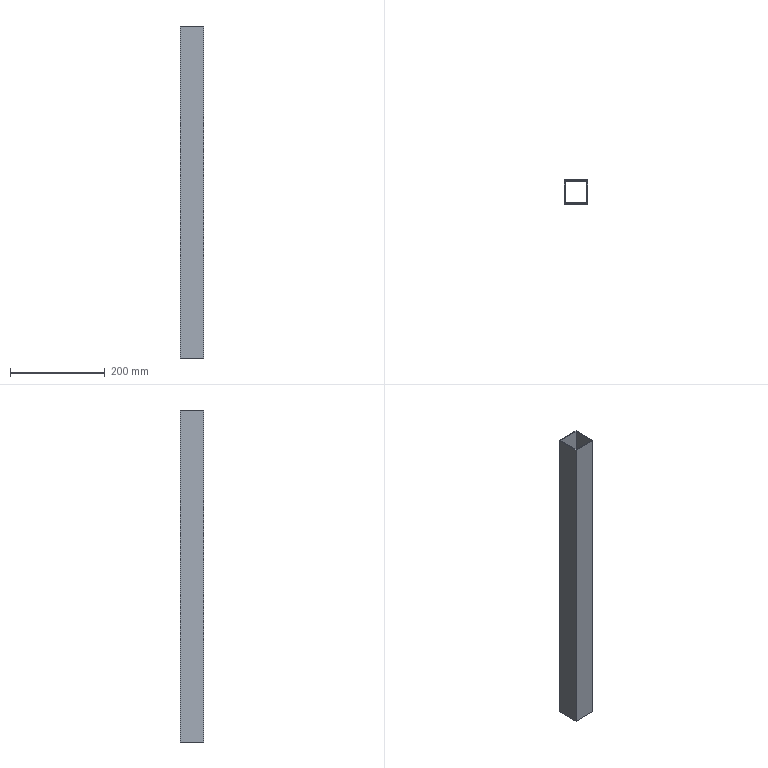Part | SolidWorks | features Extrusion 1 | 1 solid | 10 faces | box 50 x 50 x 700 mm | volume 268800 mm3 | plane 10
STEP:
#1=CARTESIAN_POINT('',(25.,-25.,700.));
#2=VERTEX_POINT('',#1);
#3=CARTESIAN_POINT('',(25.,25.,700.));
#4=VERTEX_POINT('',#3);
#5=CARTESIAN_POINT('',(25.,-25.,700.));
#6=DIRECTION('',(0.,1.,0.));
#7=VECTOR('',#6,1000.);
#8=LINE('',#5,#7);
#9=EDGE_CURVE('',#2,#4,#8,.T.);
#10=ORIENTED_EDGE('',*,*,#9,.T.);
#11=CARTESIAN_POINT('',(-25.,25.,700.));
#12=VERTEX_POINT('',#11);
#13=CARTESIAN_POINT('',(-25.,25.,700.));
#14=DIRECTION('',(-1.,0.,0.));
#15=VECTOR('',#14,1000.);
#16=LINE('',#13,#15);
#17=EDGE_CURVE('',#4,#12,#16,.T.);
#18=ORIENTED_EDGE('',*,*,#17,.T.);
#19=CARTESIAN_POINT('',(-25.,-25.,700.));
#20=VERTEX_POINT('',#19);
#21=CARTESIAN_POINT('',(-25.,-25.,700.));
#22=DIRECTION('',(0.,-1.,0.));
#23=VECTOR('',#22,1000.);
#24=LINE('',#21,#23);
#25=EDGE_CURVE('',#12,#20,#24,.T.);
#26=ORIENTED_EDGE('',*,*,#25,.T.);
#27=CARTESIAN_POINT('',(-25.,-25.,700.));
#28=DIRECTION('',(1.,0.,0.));
#29=VECTOR('',#28,1000.);
#30=LINE('',#27,#29);
#31=EDGE_CURVE('',#20,#2,#30,.T.);
#32=ORIENTED_EDGE('',*,*,#31,.T.);
#33=EDGE_LOOP('',(#10,#18,#26,#32));
#34=FACE_OUTER_BOUND('',#33,.T.);
#35=CARTESIAN_POINT('',(23.,-23.,700.));
#36=VERTEX_POINT('',#35);
#37=CARTESIAN_POINT('',(23.,23.,700.));
#38=VERTEX_POINT('',#37);
#39=CARTESIAN_POINT('',(23.,-23.,700.));
#40=DIRECTION('',(0.,1.,0.));
#41=VECTOR('',#40,1000.);
#42=LINE('',#39,#41);
#43=EDGE_CURVE('',#36,#38,#42,.T.);
#44=ORIENTED_EDGE('',*,*,#43,.F.);
#45=CARTESIAN_POINT('',(-23.,-23.,700.));
#46=VERTEX_POINT('',#45);
#47=CARTESIAN_POINT('',(-23.,-23.,700.));
#48=DIRECTION('',(1.,0.,0.));
#49=VECTOR('',#48,1000.);
#50=LINE('',#47,#49);
#51=EDGE_CURVE('',#46,#36,#50,.T.);
#52=ORIENTED_EDGE('',*,*,#51,.F.);
#53=CARTESIAN_POINT('',(-23.,23.,700.));
#54=VERTEX_POINT('',#53);
#55=CARTESIAN_POINT('',(-23.,-23.,700.));
#56=DIRECTION('',(0.,-1.,0.));
#57=VECTOR('',#56,1000.);
#58=LINE('',#55,#57);
#59=EDGE_CURVE('',#54,#46,#58,.T.);
#60=ORIENTED_EDGE('',*,*,#59,.F.);
#61=CARTESIAN_POINT('',(-23.,23.,700.));
#62=DIRECTION('',(-1.,0.,0.));
#63=VECTOR('',#62,1000.);
#64=LINE('',#61,#63);
#65=EDGE_CURVE('',#38,#54,#64,.T.);
#66=ORIENTED_EDGE('',*,*,#65,.F.);
#67=EDGE_LOOP('',(#44,#52,#60,#66));
#68=FACE_BOUND('',#67,.T.);
#69=CARTESIAN_POINT('',(0.,0.,700.));
#70=DIRECTION('',(0.,0.,-1.));
#71=DIRECTION('',(-1.,0.,0.));
#72=AXIS2_PLACEMENT_3D('',#69,#70,#71);
#73=PLANE('',#72);
#74=ADVANCED_FACE('',(#34,#68),#73,.F.);
#75=CARTESIAN_POINT('',(25.,-25.,0.));
#76=VERTEX_POINT('',#75);
#77=CARTESIAN_POINT('',(25.,25.,0.));
#78=VERTEX_POINT('',#77);
#79=CARTESIAN_POINT('',(25.,-25.,0.));
#80=DIRECTION('',(0.,1.,0.));
#81=VECTOR('',#80,1000.);
#82=LINE('',#79,#81);
#83=EDGE_CURVE('',#76,#78,#82,.T.);
#84=ORIENTED_EDGE('',*,*,#83,.F.);
#85=CARTESIAN_POINT('',(-25.,-25.,0.));
#86=VERTEX_POINT('',#85);
#87=CARTESIAN_POINT('',(-25.,-25.,0.));
#88=DIRECTION('',(1.,0.,0.));
#89=VECTOR('',#88,1000.);
#90=LINE('',#87,#89);
#91=EDGE_CURVE('',#86,#76,#90,.T.);
#92=ORIENTED_EDGE('',*,*,#91,.F.);
#93=CARTESIAN_POINT('',(-25.,25.,0.));
#94=VERTEX_POINT('',#93);
#95=CARTESIAN_POINT('',(-25.,-25.,0.));
#96=DIRECTION('',(0.,-1.,0.));
#97=VECTOR('',#96,1000.);
#98=LINE('',#95,#97);
#99=EDGE_CURVE('',#94,#86,#98,.T.);
#100=ORIENTED_EDGE('',*,*,#99,.F.);
#101=CARTESIAN_POINT('',(-25.,25.,0.));
#102=DIRECTION('',(-1.,0.,0.));
#103=VECTOR('',#102,1000.);
#104=LINE('',#101,#103);
#105=EDGE_CURVE('',#78,#94,#104,.T.);
#106=ORIENTED_EDGE('',*,*,#105,.F.);
#107=EDGE_LOOP('',(#84,#92,#100,#106));
#108=FACE_OUTER_BOUND('',#107,.T.);
#109=CARTESIAN_POINT('',(-23.,-23.,0.));
#110=VERTEX_POINT('',#109);
#111=CARTESIAN_POINT('',(23.,-23.,0.));
#112=VERTEX_POINT('',#111);
#113=CARTESIAN_POINT('',(-23.,-23.,0.));
#114=DIRECTION('',(1.,0.,0.));
#115=VECTOR('',#114,1000.);
#116=LINE('',#113,#115);
#117=EDGE_CURVE('',#110,#112,#116,.T.);
#118=ORIENTED_EDGE('',*,*,#117,.T.);
#119=CARTESIAN_POINT('',(23.,23.,0.));
#120=VERTEX_POINT('',#119);
#121=CARTESIAN_POINT('',(23.,-23.,0.));
#122=DIRECTION('',(0.,1.,0.));
#123=VECTOR('',#122,1000.);
#124=LINE('',#121,#123);
#125=EDGE_CURVE('',#112,#120,#124,.T.);
#126=ORIENTED_EDGE('',*,*,#125,.T.);
#127=CARTESIAN_POINT('',(-23.,23.,0.));
#128=VERTEX_POINT('',#127);
#129=CARTESIAN_POINT('',(-23.,23.,0.));
#130=DIRECTION('',(-1.,0.,0.));
#131=VECTOR('',#130,1000.);
#132=LINE('',#129,#131);
#133=EDGE_CURVE('',#120,#128,#132,.T.);
#134=ORIENTED_EDGE('',*,*,#133,.T.);
#135=CARTESIAN_POINT('',(-23.,-23.,0.));
#136=DIRECTION('',(0.,-1.,0.));
#137=VECTOR('',#136,1000.);
#138=LINE('',#135,#137);
#139=EDGE_CURVE('',#128,#110,#138,.T.);
#140=ORIENTED_EDGE('',*,*,#139,.T.);
#141=EDGE_LOOP('',(#118,#126,#134,#140));
#142=FACE_BOUND('',#141,.T.);
#143=CARTESIAN_POINT('',(0.,0.,0.));
#144=DIRECTION('',(0.,0.,-1.));
#145=DIRECTION('',(-1.,0.,0.));
#146=AXIS2_PLACEMENT_3D('',#143,#144,#145);
#147=PLANE('',#146);
#148=ADVANCED_FACE('',(#108,#142),#147,.T.);
#149=ORIENTED_EDGE('',*,*,#83,.T.);
#150=CARTESIAN_POINT('',(25.,25.,700.));
#151=DIRECTION('',(0.,0.,-1.));
#152=VECTOR('',#151,1000.);
#153=LINE('',#150,#152);
#154=EDGE_CURVE('',#4,#78,#153,.T.);
#155=ORIENTED_EDGE('',*,*,#154,.F.);
#156=ORIENTED_EDGE('',*,*,#9,.F.);
#157=CARTESIAN_POINT('',(25.,-25.,700.));
#158=DIRECTION('',(0.,0.,-1.));
#159=VECTOR('',#158,1000.);
#160=LINE('',#157,#159);
#161=EDGE_CURVE('',#2,#76,#160,.T.);
#162=ORIENTED_EDGE('',*,*,#161,.T.);
#163=EDGE_LOOP('',(#149,#155,#156,#162));
#164=FACE_OUTER_BOUND('',#163,.T.);
#165=CARTESIAN_POINT('',(25.,-25.,700.));
#166=DIRECTION('',(-1.,0.,0.));
#167=DIRECTION('',(0.,0.,1.));
#168=AXIS2_PLACEMENT_3D('',#165,#166,#167);
#169=PLANE('',#168);
#170=ADVANCED_FACE('',(#164),#169,.F.);
#171=ORIENTED_EDGE('',*,*,#105,.T.);
#172=CARTESIAN_POINT('',(-25.,25.,700.));
#173=DIRECTION('',(0.,0.,-1.));
#174=VECTOR('',#173,1000.);
#175=LINE('',#172,#174);
#176=EDGE_CURVE('',#12,#94,#175,.T.);
#177=ORIENTED_EDGE('',*,*,#176,.F.);
#178=ORIENTED_EDGE('',*,*,#17,.F.);
#179=ORIENTED_EDGE('',*,*,#154,.T.);
#180=EDGE_LOOP('',(#171,#177,#178,#179));
#181=FACE_OUTER_BOUND('',#180,.T.);
#182=CARTESIAN_POINT('',(-25.,25.,700.));
#183=DIRECTION('',(0.,-1.,0.));
#184=DIRECTION('',(0.,0.,-1.));
#185=AXIS2_PLACEMENT_3D('',#182,#183,#184);
#186=PLANE('',#185);
#187=ADVANCED_FACE('',(#181),#186,.F.);
#188=ORIENTED_EDGE('',*,*,#99,.T.);
#189=CARTESIAN_POINT('',(-25.,-25.,700.));
#190=DIRECTION('',(0.,0.,-1.));
#191=VECTOR('',#190,1000.);
#192=LINE('',#189,#191);
#193=EDGE_CURVE('',#20,#86,#192,.T.);
#194=ORIENTED_EDGE('',*,*,#193,.F.);
#195=ORIENTED_EDGE('',*,*,#25,.F.);
#196=ORIENTED_EDGE('',*,*,#176,.T.);
#197=EDGE_LOOP('',(#188,#194,#195,#196));
#198=FACE_OUTER_BOUND('',#197,.T.);
#199=CARTESIAN_POINT('',(-25.,-25.,700.));
#200=DIRECTION('',(1.,0.,0.));
#201=DIRECTION('',(0.,0.,-1.));
#202=AXIS2_PLACEMENT_3D('',#199,#200,#201);
#203=PLANE('',#202);
#204=ADVANCED_FACE('',(#198),#203,.F.);
#205=ORIENTED_EDGE('',*,*,#91,.T.);
#206=ORIENTED_EDGE('',*,*,#161,.F.);
#207=ORIENTED_EDGE('',*,*,#31,.F.);
#208=ORIENTED_EDGE('',*,*,#193,.T.);
#209=EDGE_LOOP('',(#205,#206,#207,#208));
#210=FACE_OUTER_BOUND('',#209,.T.);
#211=CARTESIAN_POINT('',(-25.,-25.,700.));
#212=DIRECTION('',(0.,1.,0.));
#213=DIRECTION('',(0.,0.,1.));
#214=AXIS2_PLACEMENT_3D('',#211,#212,#213);
#215=PLANE('',#214);
#216=ADVANCED_FACE('',(#210),#215,.F.);
#217=ORIENTED_EDGE('',*,*,#125,.F.);
#218=CARTESIAN_POINT('',(23.,-23.,700.));
#219=DIRECTION('',(0.,0.,-1.));
#220=VECTOR('',#219,1000.);
#221=LINE('',#218,#220);
#222=EDGE_CURVE('',#36,#112,#221,.T.);
#223=ORIENTED_EDGE('',*,*,#222,.F.);
#224=ORIENTED_EDGE('',*,*,#43,.T.);
#225=CARTESIAN_POINT('',(23.,23.,700.));
#226=DIRECTION('',(0.,0.,-1.));
#227=VECTOR('',#226,1000.);
#228=LINE('',#225,#227);
#229=EDGE_CURVE('',#38,#120,#228,.T.);
#230=ORIENTED_EDGE('',*,*,#229,.T.);
#231=EDGE_LOOP('',(#217,#223,#224,#230));
#232=FACE_OUTER_BOUND('',#231,.T.);
#233=CARTESIAN_POINT('',(23.,-23.,700.));
#234=DIRECTION('',(-1.,0.,0.));
#235=DIRECTION('',(0.,0.,1.));
#236=AXIS2_PLACEMENT_3D('',#233,#234,#235);
#237=PLANE('',#236);
#238=ADVANCED_FACE('',(#232),#237,.T.);
#239=ORIENTED_EDGE('',*,*,#133,.F.);
#240=ORIENTED_EDGE('',*,*,#229,.F.);
#241=ORIENTED_EDGE('',*,*,#65,.T.);
#242=CARTESIAN_POINT('',(-23.,23.,700.));
#243=DIRECTION('',(0.,0.,-1.));
#244=VECTOR('',#243,1000.);
#245=LINE('',#242,#244);
#246=EDGE_CURVE('',#54,#128,#245,.T.);
#247=ORIENTED_EDGE('',*,*,#246,.T.);
#248=EDGE_LOOP('',(#239,#240,#241,#247));
#249=FACE_OUTER_BOUND('',#248,.T.);
#250=CARTESIAN_POINT('',(-23.,23.,700.));
#251=DIRECTION('',(0.,-1.,0.));
#252=DIRECTION('',(0.,0.,-1.));
#253=AXIS2_PLACEMENT_3D('',#250,#251,#252);
#254=PLANE('',#253);
#255=ADVANCED_FACE('',(#249),#254,.T.);
#256=ORIENTED_EDGE('',*,*,#139,.F.);
#257=ORIENTED_EDGE('',*,*,#246,.F.);
#258=ORIENTED_EDGE('',*,*,#59,.T.);
#259=CARTESIAN_POINT('',(-23.,-23.,700.));
#260=DIRECTION('',(0.,0.,-1.));
#261=VECTOR('',#260,1000.);
#262=LINE('',#259,#261);
#263=EDGE_CURVE('',#46,#110,#262,.T.);
#264=ORIENTED_EDGE('',*,*,#263,.T.);
#265=EDGE_LOOP('',(#256,#257,#258,#264));
#266=FACE_OUTER_BOUND('',#265,.T.);
#267=CARTESIAN_POINT('',(-23.,-23.,700.));
#268=DIRECTION('',(1.,0.,0.));
#269=DIRECTION('',(0.,0.,-1.));
#270=AXIS2_PLACEMENT_3D('',#267,#268,#269);
#271=PLANE('',#270);
#272=ADVANCED_FACE('',(#266),#271,.T.);
#273=ORIENTED_EDGE('',*,*,#117,.F.);
#274=ORIENTED_EDGE('',*,*,#263,.F.);
#275=ORIENTED_EDGE('',*,*,#51,.T.);
#276=ORIENTED_EDGE('',*,*,#222,.T.);
#277=EDGE_LOOP('',(#273,#274,#275,#276));
#278=FACE_OUTER_BOUND('',#277,.T.);
#279=CARTESIAN_POINT('',(-23.,-23.,700.));
#280=DIRECTION('',(0.,1.,0.));
#281=DIRECTION('',(0.,0.,1.));
#282=AXIS2_PLACEMENT_3D('',#279,#280,#281);
#283=PLANE('',#282);
#284=ADVANCED_FACE('',(#278),#283,.T.);
#285=CLOSED_SHELL('',(#74,#148,#170,#187,#204,#216,#238,#255,#272,#284));
#286=MANIFOLD_SOLID_BREP('',#285);
#287=CARTESIAN_POINT('',(0.,0.,0.));
#288=DIRECTION('',(0.,0.,1.));
#289=DIRECTION('',(1.,0.,0.));
#290=AXIS2_PLACEMENT_3D('',#287,#288,#289);
#291=(LENGTH_UNIT()NAMED_UNIT(*)SI_UNIT(.MILLI.,.METRE.));
#292=UNCERTAINTY_MEASURE_WITH_UNIT(LENGTH_MEASURE(0.00001),#291,'','');
#293=(NAMED_UNIT(*)PLANE_ANGLE_UNIT()SI_UNIT($,.RADIAN.));
#294=(NAMED_UNIT(*)SI_UNIT($,.STERADIAN.)SOLID_ANGLE_UNIT());
#295=(GEOMETRIC_REPRESENTATION_CONTEXT(3)GLOBAL_UNCERTAINTY_ASSIGNED_CONTEXT((#292))GLOBAL_UNIT_ASSIGNED_CONTEXT((#291,#293,#294))REPRESENTATION_CONTEXT('',''));
#296=ADVANCED_BREP_SHAPE_REPRESENTATION('',(#286,#290),#295);